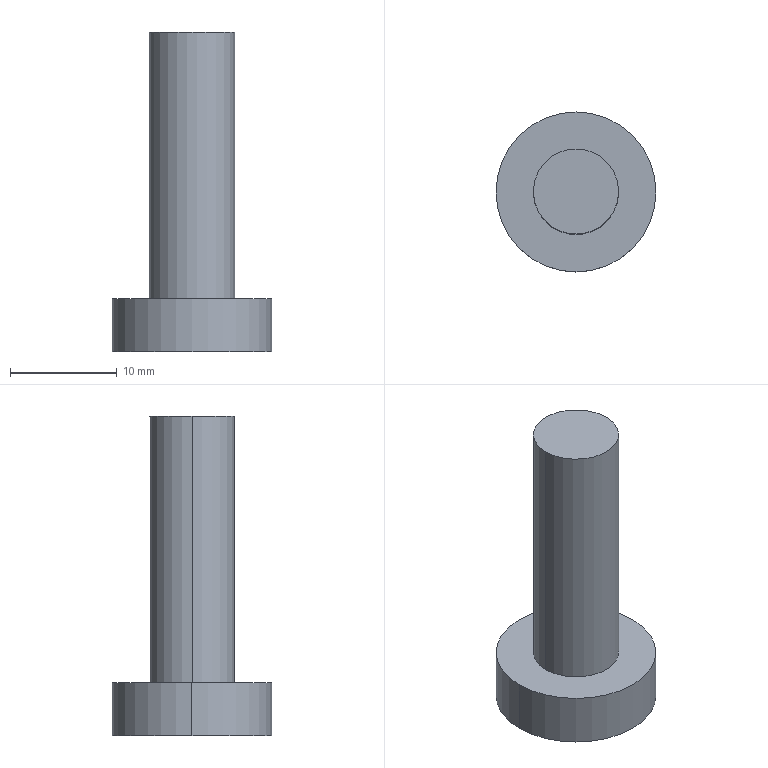Part | SolidWorks | features Extrusion 1, ICE 1 | 1 solid | 7 faces | box 15 x 15 x 30 mm | volume 2140 mm3 | cylinder 4 | plane 3 | commonest cylinder face diameters 8 x2 15 x2
STEP:
#1=CARTESIAN_POINT('',(-7.5,0.,-5.));
#2=VERTEX_POINT('',#1);
#3=CARTESIAN_POINT('',(7.5,0.,-5.));
#4=VERTEX_POINT('',#3);
#5=CARTESIAN_POINT('',(0.,0.,-5.));
#6=DIRECTION('',(0.,0.,-1.));
#7=DIRECTION('',(-1.,0.,0.));
#8=AXIS2_PLACEMENT_3D('',#5,#6,#7);
#9=CIRCLE('',#8,7.5);
#10=EDGE_CURVE('',#2,#4,#9,.T.);
#11=ORIENTED_EDGE('',*,*,#10,.F.);
#12=CARTESIAN_POINT('',(-7.5,0.,0.));
#13=VERTEX_POINT('',#12);
#14=CARTESIAN_POINT('',(-7.5,0.,-5.));
#15=DIRECTION('',(0.,0.,1.));
#16=VECTOR('',#15,1000.);
#17=LINE('',#14,#16);
#18=EDGE_CURVE('',#2,#13,#17,.T.);
#19=ORIENTED_EDGE('',*,*,#18,.T.);
#20=CARTESIAN_POINT('',(7.5,0.,0.));
#21=VERTEX_POINT('',#20);
#22=CARTESIAN_POINT('',(0.,0.,0.));
#23=DIRECTION('',(0.,0.,-1.));
#24=DIRECTION('',(-1.,0.,0.));
#25=AXIS2_PLACEMENT_3D('',#22,#23,#24);
#26=CIRCLE('',#25,7.5);
#27=EDGE_CURVE('',#13,#21,#26,.T.);
#28=ORIENTED_EDGE('',*,*,#27,.T.);
#29=CARTESIAN_POINT('',(7.5,0.,-5.));
#30=DIRECTION('',(0.,0.,1.));
#31=VECTOR('',#30,1000.);
#32=LINE('',#29,#31);
#33=EDGE_CURVE('',#4,#21,#32,.T.);
#34=ORIENTED_EDGE('',*,*,#33,.F.);
#35=EDGE_LOOP('',(#11,#19,#28,#34));
#36=FACE_OUTER_BOUND('',#35,.T.);
#37=CARTESIAN_POINT('',(0.,0.,-5.));
#38=DIRECTION('',(0.,0.,1.));
#39=DIRECTION('',(1.,0.,0.));
#40=AXIS2_PLACEMENT_3D('',#37,#38,#39);
#41=CYLINDRICAL_SURFACE('',#40,7.5);
#42=ADVANCED_FACE('',(#36),#41,.T.);
#43=CARTESIAN_POINT('',(4.,0.,25.));
#44=VERTEX_POINT('',#43);
#45=CARTESIAN_POINT('',(-4.,0.,25.));
#46=VERTEX_POINT('',#45);
#47=CARTESIAN_POINT('',(0.,0.,25.));
#48=DIRECTION('',(0.,0.,1.));
#49=DIRECTION('',(1.,0.,0.));
#50=AXIS2_PLACEMENT_3D('',#47,#48,#49);
#51=CIRCLE('',#50,4.);
#52=EDGE_CURVE('',#44,#46,#51,.T.);
#53=ORIENTED_EDGE('',*,*,#52,.F.);
#54=CARTESIAN_POINT('',(4.,0.,0.));
#55=VERTEX_POINT('',#54);
#56=CARTESIAN_POINT('',(4.,0.,25.));
#57=DIRECTION('',(0.,0.,-1.));
#58=VECTOR('',#57,1000.);
#59=LINE('',#56,#58);
#60=EDGE_CURVE('',#44,#55,#59,.T.);
#61=ORIENTED_EDGE('',*,*,#60,.T.);
#62=CARTESIAN_POINT('',(-4.,0.,0.));
#63=VERTEX_POINT('',#62);
#64=CARTESIAN_POINT('',(0.,0.,0.));
#65=DIRECTION('',(0.,0.,-1.));
#66=DIRECTION('',(-1.,0.,0.));
#67=AXIS2_PLACEMENT_3D('',#64,#65,#66);
#68=CIRCLE('',#67,4.);
#69=EDGE_CURVE('',#63,#55,#68,.T.);
#70=ORIENTED_EDGE('',*,*,#69,.F.);
#71=CARTESIAN_POINT('',(-4.,0.,25.));
#72=DIRECTION('',(0.,0.,-1.));
#73=VECTOR('',#72,1000.);
#74=LINE('',#71,#73);
#75=EDGE_CURVE('',#46,#63,#74,.T.);
#76=ORIENTED_EDGE('',*,*,#75,.F.);
#77=EDGE_LOOP('',(#53,#61,#70,#76));
#78=FACE_OUTER_BOUND('',#77,.T.);
#79=CARTESIAN_POINT('',(0.,0.,25.));
#80=DIRECTION('',(0.,0.,-1.));
#81=DIRECTION('',(-1.,0.,0.));
#82=AXIS2_PLACEMENT_3D('',#79,#80,#81);
#83=CYLINDRICAL_SURFACE('',#82,4.);
#84=ADVANCED_FACE('',(#78),#83,.T.);
#85=ORIENTED_EDGE('',*,*,#60,.F.);
#86=CARTESIAN_POINT('',(0.,0.,25.));
#87=DIRECTION('',(0.,0.,1.));
#88=DIRECTION('',(1.,0.,0.));
#89=AXIS2_PLACEMENT_3D('',#86,#87,#88);
#90=CIRCLE('',#89,4.);
#91=EDGE_CURVE('',#46,#44,#90,.T.);
#92=ORIENTED_EDGE('',*,*,#91,.F.);
#93=ORIENTED_EDGE('',*,*,#75,.T.);
#94=CARTESIAN_POINT('',(0.,0.,0.));
#95=DIRECTION('',(0.,0.,-1.));
#96=DIRECTION('',(-1.,0.,0.));
#97=AXIS2_PLACEMENT_3D('',#94,#95,#96);
#98=CIRCLE('',#97,4.);
#99=EDGE_CURVE('',#55,#63,#98,.T.);
#100=ORIENTED_EDGE('',*,*,#99,.F.);
#101=EDGE_LOOP('',(#85,#92,#93,#100));
#102=FACE_OUTER_BOUND('',#101,.T.);
#103=CARTESIAN_POINT('',(0.,0.,25.));
#104=DIRECTION('',(0.,0.,-1.));
#105=DIRECTION('',(-1.,0.,0.));
#106=AXIS2_PLACEMENT_3D('',#103,#104,#105);
#107=CYLINDRICAL_SURFACE('',#106,4.);
#108=ADVANCED_FACE('',(#102),#107,.T.);
#109=ORIENTED_EDGE('',*,*,#91,.T.);
#110=ORIENTED_EDGE('',*,*,#52,.T.);
#111=EDGE_LOOP('',(#109,#110));
#112=FACE_OUTER_BOUND('',#111,.T.);
#113=CARTESIAN_POINT('',(0.,0.,25.));
#114=DIRECTION('',(0.,0.,1.));
#115=DIRECTION('',(1.,0.,0.));
#116=AXIS2_PLACEMENT_3D('',#113,#114,#115);
#117=PLANE('',#116);
#118=ADVANCED_FACE('',(#112),#117,.T.);
#119=ORIENTED_EDGE('',*,*,#18,.F.);
#120=CARTESIAN_POINT('',(0.,0.,-5.));
#121=DIRECTION('',(0.,0.,-1.));
#122=DIRECTION('',(-1.,0.,0.));
#123=AXIS2_PLACEMENT_3D('',#120,#121,#122);
#124=CIRCLE('',#123,7.5);
#125=EDGE_CURVE('',#4,#2,#124,.T.);
#126=ORIENTED_EDGE('',*,*,#125,.F.);
#127=ORIENTED_EDGE('',*,*,#33,.T.);
#128=CARTESIAN_POINT('',(0.,0.,0.));
#129=DIRECTION('',(0.,0.,-1.));
#130=DIRECTION('',(-1.,0.,0.));
#131=AXIS2_PLACEMENT_3D('',#128,#129,#130);
#132=CIRCLE('',#131,7.5);
#133=EDGE_CURVE('',#21,#13,#132,.T.);
#134=ORIENTED_EDGE('',*,*,#133,.T.);
#135=EDGE_LOOP('',(#119,#126,#127,#134));
#136=FACE_OUTER_BOUND('',#135,.T.);
#137=CARTESIAN_POINT('',(0.,0.,-5.));
#138=DIRECTION('',(0.,0.,1.));
#139=DIRECTION('',(1.,0.,0.));
#140=AXIS2_PLACEMENT_3D('',#137,#138,#139);
#141=CYLINDRICAL_SURFACE('',#140,7.5);
#142=ADVANCED_FACE('',(#136),#141,.T.);
#143=ORIENTED_EDGE('',*,*,#125,.T.);
#144=ORIENTED_EDGE('',*,*,#10,.T.);
#145=EDGE_LOOP('',(#143,#144));
#146=FACE_OUTER_BOUND('',#145,.T.);
#147=CARTESIAN_POINT('',(0.,0.,-5.));
#148=DIRECTION('',(0.,0.,-1.));
#149=DIRECTION('',(-1.,0.,0.));
#150=AXIS2_PLACEMENT_3D('',#147,#148,#149);
#151=PLANE('',#150);
#152=ADVANCED_FACE('',(#146),#151,.T.);
#153=ORIENTED_EDGE('',*,*,#69,.T.);
#154=ORIENTED_EDGE('',*,*,#99,.T.);
#155=EDGE_LOOP('',(#153,#154));
#156=FACE_BOUND('',#155,.T.);
#157=ORIENTED_EDGE('',*,*,#133,.F.);
#158=ORIENTED_EDGE('',*,*,#27,.F.);
#159=EDGE_LOOP('',(#157,#158));
#160=FACE_OUTER_BOUND('',#159,.T.);
#161=CARTESIAN_POINT('',(0.,0.,0.));
#162=DIRECTION('',(0.,0.,-1.));
#163=DIRECTION('',(-1.,0.,0.));
#164=AXIS2_PLACEMENT_3D('',#161,#162,#163);
#165=PLANE('',#164);
#166=ADVANCED_FACE('',(#156,#160),#165,.F.);
#167=CLOSED_SHELL('',(#42,#84,#108,#118,#142,#152,#166));
#168=MANIFOLD_SOLID_BREP('',#167);
#169=CARTESIAN_POINT('',(0.,0.,0.));
#170=DIRECTION('',(0.,0.,1.));
#171=DIRECTION('',(1.,0.,0.));
#172=AXIS2_PLACEMENT_3D('',#169,#170,#171);
#173=(LENGTH_UNIT()NAMED_UNIT(*)SI_UNIT(.MILLI.,.METRE.));
#174=UNCERTAINTY_MEASURE_WITH_UNIT(LENGTH_MEASURE(0.00001),#173,'','');
#175=(NAMED_UNIT(*)PLANE_ANGLE_UNIT()SI_UNIT($,.RADIAN.));
#176=(NAMED_UNIT(*)SI_UNIT($,.STERADIAN.)SOLID_ANGLE_UNIT());
#177=(GEOMETRIC_REPRESENTATION_CONTEXT(3)GLOBAL_UNCERTAINTY_ASSIGNED_CONTEXT((#174))GLOBAL_UNIT_ASSIGNED_CONTEXT((#173,#175,#176))REPRESENTATION_CONTEXT('',''));
#178=ADVANCED_BREP_SHAPE_REPRESENTATION('',(#168,#172),#177);